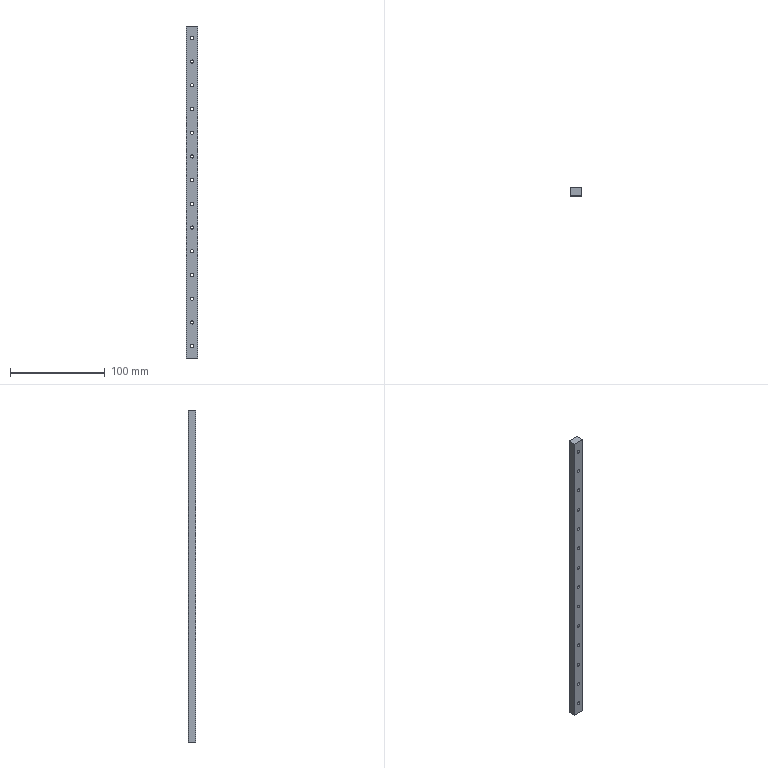Part | SolidWorks | features Chamfer 2, Extrusion 1, HoleWzd 1, LPattern 1 | 1 solid | 78 faces | box 12 x 8 x 350 mm | volume 31582 mm3 | cylinder 56 | plane 22 | commonest cylinder face diameters 3.4 x28 6 x28